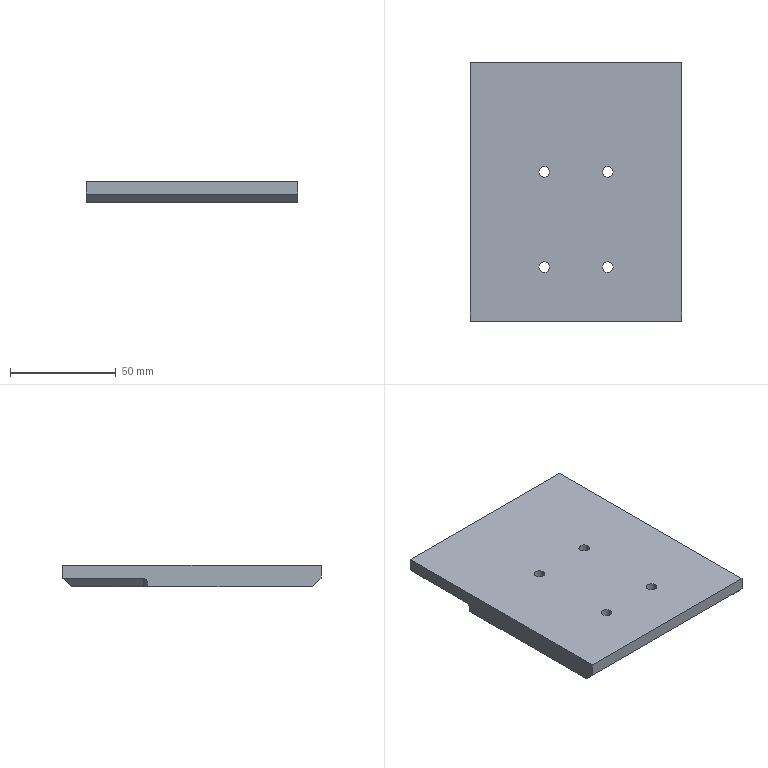Part | STEP file | X77-02102 | 1 solid | 30 faces | box 100 x 122 x 10 mm | volume 118906 mm3 | cylinder 14 | plane 12 | cone 4 | commonest cylinder face diameters 5 x8 4.2 x4 4 x2
STEP:
#1=CARTESIAN_POINT('',(17.5,9.5,10.));
#2=VERTEX_POINT('',#1);
#3=CARTESIAN_POINT('',(12.5,9.5,10.));
#4=VERTEX_POINT('',#3);
#5=CARTESIAN_POINT('',(15.,9.5,10.));
#6=DIRECTION('',(0.,0.,-1.));
#7=DIRECTION('',(-1.,0.,0.));
#8=AXIS2_PLACEMENT_3D('',#5,#6,#7);
#9=CIRCLE('',#8,2.5);
#10=EDGE_CURVE('',#2,#4,#9,.T.);
#11=ORIENTED_EDGE('',*,*,#10,.F.);
#12=CARTESIAN_POINT('',(17.5,9.5,0.));
#13=VERTEX_POINT('',#12);
#14=CARTESIAN_POINT('',(17.5,9.5,0.));
#15=DIRECTION('',(0.,0.,-1.));
#16=VECTOR('',#15,1000.);
#17=LINE('',#14,#16);
#18=EDGE_CURVE('',#2,#13,#17,.T.);
#19=ORIENTED_EDGE('',*,*,#18,.T.);
#20=CARTESIAN_POINT('',(12.5,9.5,0.));
#21=VERTEX_POINT('',#20);
#22=CARTESIAN_POINT('',(15.,9.5,0.));
#23=DIRECTION('',(0.,0.,-1.));
#24=DIRECTION('',(-1.,0.,0.));
#25=AXIS2_PLACEMENT_3D('',#22,#23,#24);
#26=CIRCLE('',#25,2.5);
#27=EDGE_CURVE('',#13,#21,#26,.T.);
#28=ORIENTED_EDGE('',*,*,#27,.T.);
#29=CARTESIAN_POINT('',(12.5,9.5,0.));
#30=DIRECTION('',(0.,0.,-1.));
#31=VECTOR('',#30,1000.);
#32=LINE('',#29,#31);
#33=EDGE_CURVE('',#4,#21,#32,.T.);
#34=ORIENTED_EDGE('',*,*,#33,.F.);
#35=EDGE_LOOP('',(#11,#19,#28,#34));
#36=FACE_OUTER_BOUND('',#35,.T.);
#37=CARTESIAN_POINT('',(15.,9.5,0.));
#38=DIRECTION('',(0.,0.,-1.));
#39=DIRECTION('',(-1.,0.,0.));
#40=AXIS2_PLACEMENT_3D('',#37,#38,#39);
#41=CYLINDRICAL_SURFACE('',#40,2.5);
#42=ADVANCED_FACE('',(#36),#41,.F.);
#43=CARTESIAN_POINT('',(17.5,-35.5,10.));
#44=VERTEX_POINT('',#43);
#45=CARTESIAN_POINT('',(12.5,-35.5,10.));
#46=VERTEX_POINT('',#45);
#47=CARTESIAN_POINT('',(15.,-35.5,10.));
#48=DIRECTION('',(0.,0.,-1.));
#49=DIRECTION('',(-1.,0.,0.));
#50=AXIS2_PLACEMENT_3D('',#47,#48,#49);
#51=CIRCLE('',#50,2.5);
#52=EDGE_CURVE('',#44,#46,#51,.T.);
#53=ORIENTED_EDGE('',*,*,#52,.F.);
#54=CARTESIAN_POINT('',(17.5,-35.5,0.));
#55=VERTEX_POINT('',#54);
#56=CARTESIAN_POINT('',(17.5,-35.5,0.));
#57=DIRECTION('',(0.,0.,-1.));
#58=VECTOR('',#57,1000.);
#59=LINE('',#56,#58);
#60=EDGE_CURVE('',#44,#55,#59,.T.);
#61=ORIENTED_EDGE('',*,*,#60,.T.);
#62=CARTESIAN_POINT('',(12.5,-35.5,0.));
#63=VERTEX_POINT('',#62);
#64=CARTESIAN_POINT('',(15.,-35.5,0.));
#65=DIRECTION('',(0.,0.,-1.));
#66=DIRECTION('',(-1.,0.,0.));
#67=AXIS2_PLACEMENT_3D('',#64,#65,#66);
#68=CIRCLE('',#67,2.5);
#69=EDGE_CURVE('',#55,#63,#68,.T.);
#70=ORIENTED_EDGE('',*,*,#69,.T.);
#71=CARTESIAN_POINT('',(12.5,-35.5,0.));
#72=DIRECTION('',(0.,0.,-1.));
#73=VECTOR('',#72,1000.);
#74=LINE('',#71,#73);
#75=EDGE_CURVE('',#46,#63,#74,.T.);
#76=ORIENTED_EDGE('',*,*,#75,.F.);
#77=EDGE_LOOP('',(#53,#61,#70,#76));
#78=FACE_OUTER_BOUND('',#77,.T.);
#79=CARTESIAN_POINT('',(15.,-35.5,0.));
#80=DIRECTION('',(0.,0.,-1.));
#81=DIRECTION('',(-1.,0.,0.));
#82=AXIS2_PLACEMENT_3D('',#79,#80,#81);
#83=CYLINDRICAL_SURFACE('',#82,2.5);
#84=ADVANCED_FACE('',(#78),#83,.F.);
#85=CARTESIAN_POINT('',(-12.5,-35.5,10.));
#86=VERTEX_POINT('',#85);
#87=CARTESIAN_POINT('',(-17.5,-35.5,10.));
#88=VERTEX_POINT('',#87);
#89=CARTESIAN_POINT('',(-15.,-35.5,10.));
#90=DIRECTION('',(0.,0.,-1.));
#91=DIRECTION('',(-1.,0.,0.));
#92=AXIS2_PLACEMENT_3D('',#89,#90,#91);
#93=CIRCLE('',#92,2.5);
#94=EDGE_CURVE('',#86,#88,#93,.T.);
#95=ORIENTED_EDGE('',*,*,#94,.F.);
#96=CARTESIAN_POINT('',(-12.5,-35.5,0.));
#97=VERTEX_POINT('',#96);
#98=CARTESIAN_POINT('',(-12.5,-35.5,0.));
#99=DIRECTION('',(0.,0.,-1.));
#100=VECTOR('',#99,1000.);
#101=LINE('',#98,#100);
#102=EDGE_CURVE('',#86,#97,#101,.T.);
#103=ORIENTED_EDGE('',*,*,#102,.T.);
#104=CARTESIAN_POINT('',(-17.5,-35.5,0.));
#105=VERTEX_POINT('',#104);
#106=CARTESIAN_POINT('',(-15.,-35.5,0.));
#107=DIRECTION('',(0.,0.,-1.));
#108=DIRECTION('',(-1.,0.,0.));
#109=AXIS2_PLACEMENT_3D('',#106,#107,#108);
#110=CIRCLE('',#109,2.5);
#111=EDGE_CURVE('',#97,#105,#110,.T.);
#112=ORIENTED_EDGE('',*,*,#111,.T.);
#113=CARTESIAN_POINT('',(-17.5,-35.5,0.));
#114=DIRECTION('',(0.,0.,-1.));
#115=VECTOR('',#114,1000.);
#116=LINE('',#113,#115);
#117=EDGE_CURVE('',#88,#105,#116,.T.);
#118=ORIENTED_EDGE('',*,*,#117,.F.);
#119=EDGE_LOOP('',(#95,#103,#112,#118));
#120=FACE_OUTER_BOUND('',#119,.T.);
#121=CARTESIAN_POINT('',(-15.,-35.5,0.));
#122=DIRECTION('',(0.,0.,-1.));
#123=DIRECTION('',(-1.,0.,0.));
#124=AXIS2_PLACEMENT_3D('',#121,#122,#123);
#125=CYLINDRICAL_SURFACE('',#124,2.5);
#126=ADVANCED_FACE('',(#120),#125,.F.);
#127=CARTESIAN_POINT('',(-12.5,9.5,10.));
#128=VERTEX_POINT('',#127);
#129=CARTESIAN_POINT('',(-17.5,9.5,10.));
#130=VERTEX_POINT('',#129);
#131=CARTESIAN_POINT('',(-15.,9.5,10.));
#132=DIRECTION('',(0.,0.,-1.));
#133=DIRECTION('',(-1.,0.,0.));
#134=AXIS2_PLACEMENT_3D('',#131,#132,#133);
#135=CIRCLE('',#134,2.5);
#136=EDGE_CURVE('',#128,#130,#135,.T.);
#137=ORIENTED_EDGE('',*,*,#136,.F.);
#138=CARTESIAN_POINT('',(-12.5,9.5,0.));
#139=VERTEX_POINT('',#138);
#140=CARTESIAN_POINT('',(-12.5,9.5,0.));
#141=DIRECTION('',(0.,0.,-1.));
#142=VECTOR('',#141,1000.);
#143=LINE('',#140,#142);
#144=EDGE_CURVE('',#128,#139,#143,.T.);
#145=ORIENTED_EDGE('',*,*,#144,.T.);
#146=CARTESIAN_POINT('',(-17.5,9.5,0.));
#147=VERTEX_POINT('',#146);
#148=CARTESIAN_POINT('',(-15.,9.5,0.));
#149=DIRECTION('',(0.,0.,-1.));
#150=DIRECTION('',(-1.,0.,0.));
#151=AXIS2_PLACEMENT_3D('',#148,#149,#150);
#152=CIRCLE('',#151,2.5);
#153=EDGE_CURVE('',#139,#147,#152,.T.);
#154=ORIENTED_EDGE('',*,*,#153,.T.);
#155=CARTESIAN_POINT('',(-17.5,9.5,0.));
#156=DIRECTION('',(0.,0.,-1.));
#157=VECTOR('',#156,1000.);
#158=LINE('',#155,#157);
#159=EDGE_CURVE('',#130,#147,#158,.T.);
#160=ORIENTED_EDGE('',*,*,#159,.F.);
#161=EDGE_LOOP('',(#137,#145,#154,#160));
#162=FACE_OUTER_BOUND('',#161,.T.);
#163=CARTESIAN_POINT('',(-15.,9.5,0.));
#164=DIRECTION('',(0.,0.,-1.));
#165=DIRECTION('',(-1.,0.,0.));
#166=AXIS2_PLACEMENT_3D('',#163,#164,#165);
#167=CYLINDRICAL_SURFACE('',#166,2.5);
#168=ADVANCED_FACE('',(#162),#167,.F.);
#169=CARTESIAN_POINT('',(32.1,41.,3.9));
#170=VERTEX_POINT('',#169);
#171=CARTESIAN_POINT('',(27.9,41.,3.9));
#172=VERTEX_POINT('',#171);
#173=CARTESIAN_POINT('',(30.,41.,3.9));
#174=DIRECTION('',(0.,0.,-1.));
#175=DIRECTION('',(-1.,0.,0.));
#176=AXIS2_PLACEMENT_3D('',#173,#174,#175);
#177=CIRCLE('',#176,2.1);
#178=EDGE_CURVE('',#170,#172,#177,.T.);
#179=ORIENTED_EDGE('',*,*,#178,.F.);
#180=CARTESIAN_POINT('',(32.1,41.,0.));
#181=VERTEX_POINT('',#180);
#182=CARTESIAN_POINT('',(32.1,41.,-8.5));
#183=DIRECTION('',(0.,0.,-1.));
#184=VECTOR('',#183,1000.);
#185=LINE('',#182,#184);
#186=EDGE_CURVE('',#170,#181,#185,.T.);
#187=ORIENTED_EDGE('',*,*,#186,.T.);
#188=CARTESIAN_POINT('',(27.9,41.,0.));
#189=VERTEX_POINT('',#188);
#190=CARTESIAN_POINT('',(30.,41.,0.));
#191=DIRECTION('',(0.,0.,-1.));
#192=DIRECTION('',(-1.,0.,0.));
#193=AXIS2_PLACEMENT_3D('',#190,#191,#192);
#194=CIRCLE('',#193,2.1);
#195=EDGE_CURVE('',#181,#189,#194,.T.);
#196=ORIENTED_EDGE('',*,*,#195,.T.);
#197=CARTESIAN_POINT('',(27.9,41.,-8.5));
#198=DIRECTION('',(0.,0.,-1.));
#199=VECTOR('',#198,1000.);
#200=LINE('',#197,#199);
#201=EDGE_CURVE('',#172,#189,#200,.T.);
#202=ORIENTED_EDGE('',*,*,#201,.F.);
#203=EDGE_LOOP('',(#179,#187,#196,#202));
#204=FACE_OUTER_BOUND('',#203,.T.);
#205=CARTESIAN_POINT('',(30.,41.,-8.5));
#206=DIRECTION('',(0.,0.,-1.));
#207=DIRECTION('',(-1.,0.,0.));
#208=AXIS2_PLACEMENT_3D('',#205,#206,#207);
#209=CYLINDRICAL_SURFACE('',#208,2.1);
#210=ADVANCED_FACE('',(#204),#209,.F.);
#211=CARTESIAN_POINT('',(30.,41.,5.162));
#212=VERTEX_POINT('',#211);
#213=CARTESIAN_POINT('',(27.9,41.,3.9));
#214=DIRECTION('',(-0.8572,0.,-0.515));
#215=VECTOR('',#214,1000.);
#216=LINE('',#213,#215);
#217=EDGE_CURVE('',#212,#172,#216,.T.);
#218=ORIENTED_EDGE('',*,*,#217,.F.);
#219=CARTESIAN_POINT('',(32.1,41.,3.9));
#220=DIRECTION('',(0.8572,0.,-0.515));
#221=VECTOR('',#220,1000.);
#222=LINE('',#219,#221);
#223=EDGE_CURVE('',#212,#170,#222,.T.);
#224=ORIENTED_EDGE('',*,*,#223,.T.);
#225=ORIENTED_EDGE('',*,*,#178,.T.);
#226=EDGE_LOOP('',(#218,#224,#225));
#227=FACE_OUTER_BOUND('',#226,.T.);
#228=CARTESIAN_POINT('',(30.,41.,3.9));
#229=DIRECTION('',(0.,0.,-1.));
#230=DIRECTION('',(-1.,0.,0.));
#231=AXIS2_PLACEMENT_3D('',#228,#229,#230);
#232=CONICAL_SURFACE('',#231,2.1,1.03);
#233=ADVANCED_FACE('',(#227),#232,.F.);
#234=CARTESIAN_POINT('',(-27.9,41.,3.9));
#235=VERTEX_POINT('',#234);
#236=CARTESIAN_POINT('',(-32.1,41.,3.9));
#237=VERTEX_POINT('',#236);
#238=CARTESIAN_POINT('',(-30.,41.,3.9));
#239=DIRECTION('',(0.,0.,-1.));
#240=DIRECTION('',(-1.,0.,0.));
#241=AXIS2_PLACEMENT_3D('',#238,#239,#240);
#242=CIRCLE('',#241,2.1);
#243=EDGE_CURVE('',#235,#237,#242,.T.);
#244=ORIENTED_EDGE('',*,*,#243,.F.);
#245=CARTESIAN_POINT('',(-27.9,41.,0.));
#246=VERTEX_POINT('',#245);
#247=CARTESIAN_POINT('',(-27.9,41.,-8.5));
#248=DIRECTION('',(0.,0.,-1.));
#249=VECTOR('',#248,1000.);
#250=LINE('',#247,#249);
#251=EDGE_CURVE('',#235,#246,#250,.T.);
#252=ORIENTED_EDGE('',*,*,#251,.T.);
#253=CARTESIAN_POINT('',(-32.1,41.,0.));
#254=VERTEX_POINT('',#253);
#255=CARTESIAN_POINT('',(-30.,41.,0.));
#256=DIRECTION('',(0.,0.,-1.));
#257=DIRECTION('',(-1.,0.,0.));
#258=AXIS2_PLACEMENT_3D('',#255,#256,#257);
#259=CIRCLE('',#258,2.1);
#260=EDGE_CURVE('',#246,#254,#259,.T.);
#261=ORIENTED_EDGE('',*,*,#260,.T.);
#262=CARTESIAN_POINT('',(-32.1,41.,-8.5));
#263=DIRECTION('',(0.,0.,-1.));
#264=VECTOR('',#263,1000.);
#265=LINE('',#262,#264);
#266=EDGE_CURVE('',#237,#254,#265,.T.);
#267=ORIENTED_EDGE('',*,*,#266,.F.);
#268=EDGE_LOOP('',(#244,#252,#261,#267));
#269=FACE_OUTER_BOUND('',#268,.T.);
#270=CARTESIAN_POINT('',(-30.,41.,-8.5));
#271=DIRECTION('',(0.,0.,-1.));
#272=DIRECTION('',(-1.,0.,0.));
#273=AXIS2_PLACEMENT_3D('',#270,#271,#272);
#274=CYLINDRICAL_SURFACE('',#273,2.1);
#275=ADVANCED_FACE('',(#269),#274,.F.);
#276=CARTESIAN_POINT('',(-30.,41.,5.162));
#277=VERTEX_POINT('',#276);
#278=CARTESIAN_POINT('',(-32.1,41.,3.9));
#279=DIRECTION('',(-0.8572,0.,-0.515));
#280=VECTOR('',#279,1000.);
#281=LINE('',#278,#280);
#282=EDGE_CURVE('',#277,#237,#281,.T.);
#283=ORIENTED_EDGE('',*,*,#282,.F.);
#284=CARTESIAN_POINT('',(-27.9,41.,3.9));
#285=DIRECTION('',(0.8572,0.,-0.515));
#286=VECTOR('',#285,1000.);
#287=LINE('',#284,#286);
#288=EDGE_CURVE('',#277,#235,#287,.T.);
#289=ORIENTED_EDGE('',*,*,#288,.T.);
#290=ORIENTED_EDGE('',*,*,#243,.T.);
#291=EDGE_LOOP('',(#283,#289,#290));
#292=FACE_OUTER_BOUND('',#291,.T.);
#293=CARTESIAN_POINT('',(-30.,41.,3.9));
#294=DIRECTION('',(0.,0.,-1.));
#295=DIRECTION('',(-1.,0.,0.));
#296=AXIS2_PLACEMENT_3D('',#293,#294,#295);
#297=CONICAL_SURFACE('',#296,2.1,1.03);
#298=ADVANCED_FACE('',(#292),#297,.F.);
#299=CARTESIAN_POINT('',(50.,-61.,10.));
#300=VERTEX_POINT('',#299);
#301=CARTESIAN_POINT('',(50.,-61.,4.));
#302=VERTEX_POINT('',#301);
#303=CARTESIAN_POINT('',(50.,-61.,10.));
#304=DIRECTION('',(0.,0.,-1.));
#305=VECTOR('',#304,1000.);
#306=LINE('',#303,#305);
#307=EDGE_CURVE('',#300,#302,#306,.T.);
#308=ORIENTED_EDGE('',*,*,#307,.T.);
#309=CARTESIAN_POINT('',(50.,-57.,0.));
#310=VERTEX_POINT('',#309);
#311=CARTESIAN_POINT('',(50.,-61.,4.));
#312=DIRECTION('',(0.,0.7071,-0.7071));
#313=VECTOR('',#312,1000.);
#314=LINE('',#311,#313);
#315=EDGE_CURVE('',#302,#310,#314,.T.);
#316=ORIENTED_EDGE('',*,*,#315,.T.);
#317=CARTESIAN_POINT('',(50.,21.,0.));
#318=VERTEX_POINT('',#317);
#319=CARTESIAN_POINT('',(50.,-61.,0.));
#320=DIRECTION('',(0.,1.,0.));
#321=VECTOR('',#320,1000.);
#322=LINE('',#319,#321);
#323=EDGE_CURVE('',#310,#318,#322,.T.);
#324=ORIENTED_EDGE('',*,*,#323,.T.);
#325=CARTESIAN_POINT('',(50.,21.,1.172));
#326=VERTEX_POINT('',#325);
#327=CARTESIAN_POINT('',(50.,21.,4.));
#328=DIRECTION('',(0.,0.,-1.));
#329=VECTOR('',#328,1000.);
#330=LINE('',#327,#329);
#331=EDGE_CURVE('',#326,#318,#330,.T.);
#332=ORIENTED_EDGE('',*,*,#331,.F.);
#333=CARTESIAN_POINT('',(50.,23.,4.));
#334=VERTEX_POINT('',#333);
#335=CARTESIAN_POINT('',(50.,21.,1.172));
#336=CARTESIAN_POINT('',(50.,21.,2.828));
#337=CARTESIAN_POINT('',(50.,21.828,4.));
#338=CARTESIAN_POINT('',(50.,23.,4.));
#339=(BOUNDED_CURVE()B_SPLINE_CURVE(3,(#335,#336,#337,#338),.UNSPECIFIED.,.F.,.F.)B_SPLINE_CURVE_WITH_KNOTS((4,4),(4.712,6.283),.UNSPECIFIED.)CURVE()GEOMETRIC_REPRESENTATION_ITEM()RATIONAL_B_SPLINE_CURVE((1.,0.8047,0.8047,1.))REPRESENTATION_ITEM(''));
#340=EDGE_CURVE('',#326,#334,#339,.T.);
#341=ORIENTED_EDGE('',*,*,#340,.T.);
#342=CARTESIAN_POINT('',(50.,61.,4.));
#343=VERTEX_POINT('',#342);
#344=CARTESIAN_POINT('',(50.,21.,4.));
#345=DIRECTION('',(0.,1.,0.));
#346=VECTOR('',#345,1000.);
#347=LINE('',#344,#346);
#348=EDGE_CURVE('',#334,#343,#347,.T.);
#349=ORIENTED_EDGE('',*,*,#348,.T.);
#350=CARTESIAN_POINT('',(50.,61.,10.));
#351=VERTEX_POINT('',#350);
#352=CARTESIAN_POINT('',(50.,61.,10.));
#353=DIRECTION('',(0.,0.,-1.));
#354=VECTOR('',#353,1000.);
#355=LINE('',#352,#354);
#356=EDGE_CURVE('',#351,#343,#355,.T.);
#357=ORIENTED_EDGE('',*,*,#356,.F.);
#358=CARTESIAN_POINT('',(50.,-61.,10.));
#359=DIRECTION('',(0.,1.,0.));
#360=VECTOR('',#359,1000.);
#361=LINE('',#358,#360);
#362=EDGE_CURVE('',#300,#351,#361,.T.);
#363=ORIENTED_EDGE('',*,*,#362,.F.);
#364=EDGE_LOOP('',(#308,#316,#324,#332,#341,#349,#357,#363));
#365=FACE_OUTER_BOUND('',#364,.T.);
#366=CARTESIAN_POINT('',(50.,-61.,10.));
#367=DIRECTION('',(-1.,0.,0.));
#368=DIRECTION('',(0.,0.,1.));
#369=AXIS2_PLACEMENT_3D('',#366,#367,#368);
#370=PLANE('',#369);
#371=ADVANCED_FACE('',(#365),#370,.F.);
#372=ORIENTED_EDGE('',*,*,#356,.T.);
#373=CARTESIAN_POINT('',(-50.,61.,4.));
#374=VERTEX_POINT('',#373);
#375=CARTESIAN_POINT('',(-50.,61.,4.));
#376=DIRECTION('',(-1.,0.,0.));
#377=VECTOR('',#376,1000.);
#378=LINE('',#375,#377);
#379=EDGE_CURVE('',#343,#374,#378,.T.);
#380=ORIENTED_EDGE('',*,*,#379,.T.);
#381=CARTESIAN_POINT('',(-50.,61.,10.));
#382=VERTEX_POINT('',#381);
#383=CARTESIAN_POINT('',(-50.,61.,10.));
#384=DIRECTION('',(0.,0.,-1.));
#385=VECTOR('',#384,1000.);
#386=LINE('',#383,#385);
#387=EDGE_CURVE('',#382,#374,#386,.T.);
#388=ORIENTED_EDGE('',*,*,#387,.F.);
#389=CARTESIAN_POINT('',(-50.,61.,10.));
#390=DIRECTION('',(-1.,0.,0.));
#391=VECTOR('',#390,1000.);
#392=LINE('',#389,#391);
#393=EDGE_CURVE('',#351,#382,#392,.T.);
#394=ORIENTED_EDGE('',*,*,#393,.F.);
#395=EDGE_LOOP('',(#372,#380,#388,#394));
#396=FACE_OUTER_BOUND('',#395,.T.);
#397=CARTESIAN_POINT('',(-50.,61.,10.));
#398=DIRECTION('',(0.,-1.,0.));
#399=DIRECTION('',(0.,0.,-1.));
#400=AXIS2_PLACEMENT_3D('',#397,#398,#399);
#401=PLANE('',#400);
#402=ADVANCED_FACE('',(#396),#401,.F.);
#403=CARTESIAN_POINT('',(-50.,21.,0.));
#404=VERTEX_POINT('',#403);
#405=CARTESIAN_POINT('',(-50.,-57.,0.));
#406=VERTEX_POINT('',#405);
#407=CARTESIAN_POINT('',(-50.,-61.,0.));
#408=DIRECTION('',(0.,-1.,0.));
#409=VECTOR('',#408,1000.);
#410=LINE('',#407,#409);
#411=EDGE_CURVE('',#404,#406,#410,.T.);
#412=ORIENTED_EDGE('',*,*,#411,.T.);
#413=CARTESIAN_POINT('',(-50.,-61.,4.));
#414=VERTEX_POINT('',#413);
#415=CARTESIAN_POINT('',(-50.,-61.,4.));
#416=DIRECTION('',(0.,-0.7071,0.7071));
#417=VECTOR('',#416,1000.);
#418=LINE('',#415,#417);
#419=EDGE_CURVE('',#406,#414,#418,.T.);
#420=ORIENTED_EDGE('',*,*,#419,.T.);
#421=CARTESIAN_POINT('',(-50.,-61.,10.));
#422=VERTEX_POINT('',#421);
#423=CARTESIAN_POINT('',(-50.,-61.,10.));
#424=DIRECTION('',(0.,0.,-1.));
#425=VECTOR('',#424,1000.);
#426=LINE('',#423,#425);
#427=EDGE_CURVE('',#422,#414,#426,.T.);
#428=ORIENTED_EDGE('',*,*,#427,.F.);
#429=CARTESIAN_POINT('',(-50.,-61.,10.));
#430=DIRECTION('',(0.,-1.,0.));
#431=VECTOR('',#430,1000.);
#432=LINE('',#429,#431);
#433=EDGE_CURVE('',#382,#422,#432,.T.);
#434=ORIENTED_EDGE('',*,*,#433,.F.);
#435=ORIENTED_EDGE('',*,*,#387,.T.);
#436=CARTESIAN_POINT('',(-50.,23.,4.));
#437=VERTEX_POINT('',#436);
#438=CARTESIAN_POINT('',(-50.,21.,4.));
#439=DIRECTION('',(0.,1.,0.));
#440=VECTOR('',#439,1000.);
#441=LINE('',#438,#440);
#442=EDGE_CURVE('',#437,#374,#441,.T.);
#443=ORIENTED_EDGE('',*,*,#442,.F.);
#444=CARTESIAN_POINT('',(-50.,21.,1.172));
#445=VERTEX_POINT('',#444);
#446=CARTESIAN_POINT('',(-50.,23.,4.));
#447=CARTESIAN_POINT('',(-50.,21.828,4.));
#448=CARTESIAN_POINT('',(-50.,21.,2.828));
#449=CARTESIAN_POINT('',(-50.,21.,1.172));
#450=(BOUNDED_CURVE()B_SPLINE_CURVE(3,(#446,#447,#448,#449),.UNSPECIFIED.,.F.,.F.)B_SPLINE_CURVE_WITH_KNOTS((4,4),(0.,1.571),.UNSPECIFIED.)CURVE()GEOMETRIC_REPRESENTATION_ITEM()RATIONAL_B_SPLINE_CURVE((1.,0.8047,0.8047,1.))REPRESENTATION_ITEM(''));
#451=EDGE_CURVE('',#437,#445,#450,.T.);
#452=ORIENTED_EDGE('',*,*,#451,.T.);
#453=CARTESIAN_POINT('',(-50.,21.,0.));
#454=DIRECTION('',(0.,0.,1.));
#455=VECTOR('',#454,1000.);
#456=LINE('',#453,#455);
#457=EDGE_CURVE('',#404,#445,#456,.T.);
#458=ORIENTED_EDGE('',*,*,#457,.F.);
#459=EDGE_LOOP('',(#412,#420,#428,#434,#435,#443,#452,#458));
#460=FACE_OUTER_BOUND('',#459,.T.);
#461=CARTESIAN_POINT('',(-50.,-61.,10.));
#462=DIRECTION('',(1.,0.,0.));
#463=DIRECTION('',(0.,0.,-1.));
#464=AXIS2_PLACEMENT_3D('',#461,#462,#463);
#465=PLANE('',#464);
#466=ADVANCED_FACE('',(#460),#465,.F.);
#467=ORIENTED_EDGE('',*,*,#427,.T.);
#468=CARTESIAN_POINT('',(50.,-61.,4.));
#469=DIRECTION('',(1.,0.,0.));
#470=VECTOR('',#469,1000.);
#471=LINE('',#468,#470);
#472=EDGE_CURVE('',#414,#302,#471,.T.);
#473=ORIENTED_EDGE('',*,*,#472,.T.);
#474=ORIENTED_EDGE('',*,*,#307,.F.);
#475=CARTESIAN_POINT('',(-50.,-61.,10.));
#476=DIRECTION('',(1.,0.,0.));
#477=VECTOR('',#476,1000.);
#478=LINE('',#475,#477);
#479=EDGE_CURVE('',#422,#300,#478,.T.);
#480=ORIENTED_EDGE('',*,*,#479,.F.);
#481=EDGE_LOOP('',(#467,#473,#474,#480));
#482=FACE_OUTER_BOUND('',#481,.T.);
#483=CARTESIAN_POINT('',(-50.,-61.,10.));
#484=DIRECTION('',(0.,1.,0.));
#485=DIRECTION('',(0.,0.,1.));
#486=AXIS2_PLACEMENT_3D('',#483,#484,#485);
#487=PLANE('',#486);
#488=ADVANCED_FACE('',(#482),#487,.F.);
#489=CARTESIAN_POINT('',(15.,9.5,10.));
#490=DIRECTION('',(0.,0.,-1.));
#491=DIRECTION('',(-1.,0.,0.));
#492=AXIS2_PLACEMENT_3D('',#489,#490,#491);
#493=CIRCLE('',#492,2.5);
#494=EDGE_CURVE('',#4,#2,#493,.T.);
#495=ORIENTED_EDGE('',*,*,#494,.T.);
#496=ORIENTED_EDGE('',*,*,#10,.T.);
#497=EDGE_LOOP('',(#495,#496));
#498=FACE_BOUND('',#497,.T.);
#499=CARTESIAN_POINT('',(15.,-35.5,10.));
#500=DIRECTION('',(0.,0.,-1.));
#501=DIRECTION('',(-1.,0.,0.));
#502=AXIS2_PLACEMENT_3D('',#499,#500,#501);
#503=CIRCLE('',#502,2.5);
#504=EDGE_CURVE('',#46,#44,#503,.T.);
#505=ORIENTED_EDGE('',*,*,#504,.T.);
#506=ORIENTED_EDGE('',*,*,#52,.T.);
#507=EDGE_LOOP('',(#505,#506));
#508=FACE_BOUND('',#507,.T.);
#509=CARTESIAN_POINT('',(-15.,-35.5,10.));
#510=DIRECTION('',(0.,0.,-1.));
#511=DIRECTION('',(-1.,0.,0.));
#512=AXIS2_PLACEMENT_3D('',#509,#510,#511);
#513=CIRCLE('',#512,2.5);
#514=EDGE_CURVE('',#88,#86,#513,.T.);
#515=ORIENTED_EDGE('',*,*,#514,.T.);
#516=ORIENTED_EDGE('',*,*,#94,.T.);
#517=EDGE_LOOP('',(#515,#516));
#518=FACE_BOUND('',#517,.T.);
#519=CARTESIAN_POINT('',(-15.,9.5,10.));
#520=DIRECTION('',(0.,0.,-1.));
#521=DIRECTION('',(-1.,0.,0.));
#522=AXIS2_PLACEMENT_3D('',#519,#520,#521);
#523=CIRCLE('',#522,2.5);
#524=EDGE_CURVE('',#130,#128,#523,.T.);
#525=ORIENTED_EDGE('',*,*,#524,.T.);
#526=ORIENTED_EDGE('',*,*,#136,.T.);
#527=EDGE_LOOP('',(#525,#526));
#528=FACE_BOUND('',#527,.T.);
#529=ORIENTED_EDGE('',*,*,#362,.T.);
#530=ORIENTED_EDGE('',*,*,#393,.T.);
#531=ORIENTED_EDGE('',*,*,#433,.T.);
#532=ORIENTED_EDGE('',*,*,#479,.T.);
#533=EDGE_LOOP('',(#529,#530,#531,#532));
#534=FACE_OUTER_BOUND('',#533,.T.);
#535=CARTESIAN_POINT('',(50.,61.,10.));
#536=DIRECTION('',(0.,0.,-1.));
#537=DIRECTION('',(-1.,0.,0.));
#538=AXIS2_PLACEMENT_3D('',#535,#536,#537);
#539=PLANE('',#538);
#540=ADVANCED_FACE('',(#498,#508,#518,#528,#534),#539,.F.);
#541=CARTESIAN_POINT('',(15.,9.5,0.));
#542=DIRECTION('',(0.,0.,-1.));
#543=DIRECTION('',(-1.,0.,0.));
#544=AXIS2_PLACEMENT_3D('',#541,#542,#543);
#545=CIRCLE('',#544,2.5);
#546=EDGE_CURVE('',#21,#13,#545,.T.);
#547=ORIENTED_EDGE('',*,*,#546,.F.);
#548=ORIENTED_EDGE('',*,*,#27,.F.);
#549=EDGE_LOOP('',(#547,#548));
#550=FACE_BOUND('',#549,.T.);
#551=CARTESIAN_POINT('',(15.,-35.5,0.));
#552=DIRECTION('',(0.,0.,-1.));
#553=DIRECTION('',(-1.,0.,0.));
#554=AXIS2_PLACEMENT_3D('',#551,#552,#553);
#555=CIRCLE('',#554,2.5);
#556=EDGE_CURVE('',#63,#55,#555,.T.);
#557=ORIENTED_EDGE('',*,*,#556,.F.);
#558=ORIENTED_EDGE('',*,*,#69,.F.);
#559=EDGE_LOOP('',(#557,#558));
#560=FACE_BOUND('',#559,.T.);
#561=CARTESIAN_POINT('',(-15.,-35.5,0.));
#562=DIRECTION('',(0.,0.,-1.));
#563=DIRECTION('',(-1.,0.,0.));
#564=AXIS2_PLACEMENT_3D('',#561,#562,#563);
#565=CIRCLE('',#564,2.5);
#566=EDGE_CURVE('',#105,#97,#565,.T.);
#567=ORIENTED_EDGE('',*,*,#566,.F.);
#568=ORIENTED_EDGE('',*,*,#111,.F.);
#569=EDGE_LOOP('',(#567,#568));
#570=FACE_BOUND('',#569,.T.);
#571=CARTESIAN_POINT('',(-15.,9.5,0.));
#572=DIRECTION('',(0.,0.,-1.));
#573=DIRECTION('',(-1.,0.,0.));
#574=AXIS2_PLACEMENT_3D('',#571,#572,#573);
#575=CIRCLE('',#574,2.5);
#576=EDGE_CURVE('',#147,#139,#575,.T.);
#577=ORIENTED_EDGE('',*,*,#576,.F.);
#578=ORIENTED_EDGE('',*,*,#153,.F.);
#579=EDGE_LOOP('',(#577,#578));
#580=FACE_BOUND('',#579,.T.);
#581=CARTESIAN_POINT('',(30.,41.,0.));
#582=DIRECTION('',(0.,0.,-1.));
#583=DIRECTION('',(-1.,0.,0.));
#584=AXIS2_PLACEMENT_3D('',#581,#582,#583);
#585=CIRCLE('',#584,2.1);
#586=EDGE_CURVE('',#189,#181,#585,.T.);
#587=ORIENTED_EDGE('',*,*,#586,.F.);
#588=ORIENTED_EDGE('',*,*,#195,.F.);
#589=EDGE_LOOP('',(#587,#588));
#590=FACE_BOUND('',#589,.T.);
#591=CARTESIAN_POINT('',(-30.,41.,0.));
#592=DIRECTION('',(0.,0.,-1.));
#593=DIRECTION('',(-1.,0.,0.));
#594=AXIS2_PLACEMENT_3D('',#591,#592,#593);
#595=CIRCLE('',#594,2.1);
#596=EDGE_CURVE('',#254,#246,#595,.T.);
#597=ORIENTED_EDGE('',*,*,#596,.F.);
#598=ORIENTED_EDGE('',*,*,#260,.F.);
#599=EDGE_LOOP('',(#597,#598));
#600=FACE_BOUND('',#599,.T.);
#601=ORIENTED_EDGE('',*,*,#323,.F.);
#602=CARTESIAN_POINT('',(-50.,-57.,0.));
#603=DIRECTION('',(-1.,0.,0.));
#604=VECTOR('',#603,1000.);
#605=LINE('',#602,#604);
#606=EDGE_CURVE('',#310,#406,#605,.T.);
#607=ORIENTED_EDGE('',*,*,#606,.T.);
#608=ORIENTED_EDGE('',*,*,#411,.F.);
#609=CARTESIAN_POINT('',(-48.828,21.,0.));
#610=VERTEX_POINT('',#609);
#611=CARTESIAN_POINT('',(-46.,21.,0.));
#612=DIRECTION('',(-1.,0.,0.));
#613=VECTOR('',#612,1000.);
#614=LINE('',#611,#613);
#615=EDGE_CURVE('',#610,#404,#614,.T.);
#616=ORIENTED_EDGE('',*,*,#615,.F.);
#617=CARTESIAN_POINT('',(-46.,23.,0.));
#618=VERTEX_POINT('',#617);
#619=CARTESIAN_POINT('',(-48.828,21.,0.));
#620=CARTESIAN_POINT('',(-47.172,21.,0.));
#621=CARTESIAN_POINT('',(-46.,21.828,0.));
#622=CARTESIAN_POINT('',(-46.,23.,0.));
#623=(BOUNDED_CURVE()B_SPLINE_CURVE(3,(#619,#620,#621,#622),.UNSPECIFIED.,.F.,.F.)B_SPLINE_CURVE_WITH_KNOTS((4,4),(1.571,3.142),.UNSPECIFIED.)CURVE()GEOMETRIC_REPRESENTATION_ITEM()RATIONAL_B_SPLINE_CURVE((1.,0.8047,0.8047,1.))REPRESENTATION_ITEM(''));
#624=EDGE_CURVE('',#610,#618,#623,.T.);
#625=ORIENTED_EDGE('',*,*,#624,.T.);
#626=CARTESIAN_POINT('',(-46.,57.,0.));
#627=VERTEX_POINT('',#626);
#628=CARTESIAN_POINT('',(-46.,21.,0.));
#629=DIRECTION('',(0.,1.,0.));
#630=VECTOR('',#629,1000.);
#631=LINE('',#628,#630);
#632=EDGE_CURVE('',#618,#627,#631,.T.);
#633=ORIENTED_EDGE('',*,*,#632,.T.);
#634=CARTESIAN_POINT('',(46.,57.,0.));
#635=VERTEX_POINT('',#634);
#636=CARTESIAN_POINT('',(50.,57.,0.));
#637=DIRECTION('',(1.,0.,0.));
#638=VECTOR('',#637,1000.);
#639=LINE('',#636,#638);
#640=EDGE_CURVE('',#627,#635,#639,.T.);
#641=ORIENTED_EDGE('',*,*,#640,.T.);
#642=CARTESIAN_POINT('',(46.,23.,0.));
#643=VERTEX_POINT('',#642);
#644=CARTESIAN_POINT('',(46.,21.,0.));
#645=DIRECTION('',(0.,1.,0.));
#646=VECTOR('',#645,1000.);
#647=LINE('',#644,#646);
#648=EDGE_CURVE('',#643,#635,#647,.T.);
#649=ORIENTED_EDGE('',*,*,#648,.F.);
#650=CARTESIAN_POINT('',(48.828,21.,0.));
#651=VERTEX_POINT('',#650);
#652=CARTESIAN_POINT('',(46.,23.,0.));
#653=CARTESIAN_POINT('',(46.,21.828,0.));
#654=CARTESIAN_POINT('',(47.172,21.,0.));
#655=CARTESIAN_POINT('',(48.828,21.,0.));
#656=(BOUNDED_CURVE()B_SPLINE_CURVE(3,(#652,#653,#654,#655),.UNSPECIFIED.,.F.,.F.)B_SPLINE_CURVE_WITH_KNOTS((4,4),(3.142,4.712),.UNSPECIFIED.)CURVE()GEOMETRIC_REPRESENTATION_ITEM()RATIONAL_B_SPLINE_CURVE((1.,0.8047,0.8047,1.))REPRESENTATION_ITEM(''));
#657=EDGE_CURVE('',#643,#651,#656,.T.);
#658=ORIENTED_EDGE('',*,*,#657,.T.);
#659=CARTESIAN_POINT('',(50.,21.,0.));
#660=DIRECTION('',(-1.,0.,0.));
#661=VECTOR('',#660,1000.);
#662=LINE('',#659,#661);
#663=EDGE_CURVE('',#318,#651,#662,.T.);
#664=ORIENTED_EDGE('',*,*,#663,.F.);
#665=EDGE_LOOP('',(#601,#607,#608,#616,#625,#633,#641,#649,#658,#664));
#666=FACE_OUTER_BOUND('',#665,.T.);
#667=CARTESIAN_POINT('',(50.,61.,0.));
#668=DIRECTION('',(0.,0.,-1.));
#669=DIRECTION('',(-1.,0.,0.));
#670=AXIS2_PLACEMENT_3D('',#667,#668,#669);
#671=PLANE('',#670);
#672=ADVANCED_FACE('',(#550,#560,#570,#580,#590,#600,#666),#671,.T.);
#673=CARTESIAN_POINT('',(16.667,27.667,-29.333));
#674=DIRECTION('',(0.5774,0.5774,0.5774));
#675=VECTOR('',#674,1000.);
#676=LINE('',#673,#675);
#677=EDGE_CURVE('',#635,#343,#676,.T.);
#678=ORIENTED_EDGE('',*,*,#677,.F.);
#679=ORIENTED_EDGE('',*,*,#640,.F.);
#680=CARTESIAN_POINT('',(-50.,61.,4.));
#681=DIRECTION('',(0.5774,-0.5774,-0.5774));
#682=VECTOR('',#681,1000.);
#683=LINE('',#680,#682);
#684=EDGE_CURVE('',#374,#627,#683,.T.);
#685=ORIENTED_EDGE('',*,*,#684,.F.);
#686=ORIENTED_EDGE('',*,*,#379,.F.);
#687=EDGE_LOOP('',(#678,#679,#685,#686));
#688=FACE_OUTER_BOUND('',#687,.T.);
#689=CARTESIAN_POINT('',(-50.,61.,4.));
#690=DIRECTION('',(0.,0.7071,-0.7071));
#691=DIRECTION('',(0.,0.7071,0.7071));
#692=AXIS2_PLACEMENT_3D('',#689,#690,#691);
#693=PLANE('',#692);
#694=ADVANCED_FACE('',(#688),#693,.T.);
#695=ORIENTED_EDGE('',*,*,#632,.F.);
#696=CARTESIAN_POINT('',(-50.,23.,4.));
#697=DIRECTION('',(-0.7071,0.,0.7071));
#698=VECTOR('',#697,1000.);
#699=LINE('',#696,#698);
#700=EDGE_CURVE('',#618,#437,#699,.T.);
#701=ORIENTED_EDGE('',*,*,#700,.T.);
#702=ORIENTED_EDGE('',*,*,#442,.T.);
#703=ORIENTED_EDGE('',*,*,#684,.T.);
#704=EDGE_LOOP('',(#695,#701,#702,#703));
#705=FACE_OUTER_BOUND('',#704,.T.);
#706=CARTESIAN_POINT('',(-50.,21.,4.));
#707=DIRECTION('',(0.7071,0.,0.7071));
#708=DIRECTION('',(0.7071,0.,-0.7071));
#709=AXIS2_PLACEMENT_3D('',#706,#707,#708);
#710=PLANE('',#709);
#711=ADVANCED_FACE('',(#705),#710,.F.);
#712=ORIENTED_EDGE('',*,*,#457,.T.);
#713=CARTESIAN_POINT('',(-47.414,21.,-1.414));
#714=DIRECTION('',(0.7071,0.,-0.7071));
#715=VECTOR('',#714,1000.);
#716=LINE('',#713,#715);
#717=EDGE_CURVE('',#445,#610,#716,.T.);
#718=ORIENTED_EDGE('',*,*,#717,.T.);
#719=ORIENTED_EDGE('',*,*,#615,.T.);
#720=EDGE_LOOP('',(#712,#718,#719));
#721=FACE_OUTER_BOUND('',#720,.T.);
#722=CARTESIAN_POINT('',(-50.,21.,0.));
#723=DIRECTION('',(0.,-1.,0.));
#724=DIRECTION('',(0.,0.,-1.));
#725=AXIS2_PLACEMENT_3D('',#722,#723,#724);
#726=PLANE('',#725);
#727=ADVANCED_FACE('',(#721),#726,.F.);
#728=ORIENTED_EDGE('',*,*,#348,.F.);
#729=CARTESIAN_POINT('',(46.,23.,0.));
#730=DIRECTION('',(-0.7071,0.,-0.7071));
#731=VECTOR('',#730,1000.);
#732=LINE('',#729,#731);
#733=EDGE_CURVE('',#334,#643,#732,.T.);
#734=ORIENTED_EDGE('',*,*,#733,.T.);
#735=ORIENTED_EDGE('',*,*,#648,.T.);
#736=ORIENTED_EDGE('',*,*,#677,.T.);
#737=EDGE_LOOP('',(#728,#734,#735,#736));
#738=FACE_OUTER_BOUND('',#737,.T.);
#739=CARTESIAN_POINT('',(46.,21.,0.));
#740=DIRECTION('',(-0.7071,0.,0.7071));
#741=DIRECTION('',(0.7071,0.,0.7071));
#742=AXIS2_PLACEMENT_3D('',#739,#740,#741);
#743=PLANE('',#742);
#744=ADVANCED_FACE('',(#738),#743,.F.);
#745=ORIENTED_EDGE('',*,*,#663,.T.);
#746=CARTESIAN_POINT('',(51.414,21.,2.586));
#747=DIRECTION('',(0.7071,0.,0.7071));
#748=VECTOR('',#747,1000.);
#749=LINE('',#746,#748);
#750=EDGE_CURVE('',#651,#326,#749,.T.);
#751=ORIENTED_EDGE('',*,*,#750,.T.);
#752=ORIENTED_EDGE('',*,*,#331,.T.);
#753=EDGE_LOOP('',(#745,#751,#752));
#754=FACE_OUTER_BOUND('',#753,.T.);
#755=CARTESIAN_POINT('',(50.,21.,4.));
#756=DIRECTION('',(0.,1.,0.));
#757=DIRECTION('',(0.,0.,1.));
#758=AXIS2_PLACEMENT_3D('',#755,#756,#757);
#759=PLANE('',#758);
#760=ADVANCED_FACE('',(#754),#759,.T.);
#761=ORIENTED_EDGE('',*,*,#451,.F.);
#762=ORIENTED_EDGE('',*,*,#700,.F.);
#763=ORIENTED_EDGE('',*,*,#624,.F.);
#764=ORIENTED_EDGE('',*,*,#717,.F.);
#765=EDGE_LOOP('',(#761,#762,#763,#764));
#766=FACE_OUTER_BOUND('',#765,.T.);
#767=CARTESIAN_POINT('',(-49.414,23.,0.5858));
#768=DIRECTION('',(-0.7071,0.,0.7071));
#769=DIRECTION('',(0.7071,0.,0.7071));
#770=AXIS2_PLACEMENT_3D('',#767,#768,#769);
#771=CYLINDRICAL_SURFACE('',#770,2.);
#772=ADVANCED_FACE('',(#766),#771,.F.);
#773=ORIENTED_EDGE('',*,*,#657,.F.);
#774=ORIENTED_EDGE('',*,*,#733,.F.);
#775=ORIENTED_EDGE('',*,*,#340,.F.);
#776=ORIENTED_EDGE('',*,*,#750,.F.);
#777=EDGE_LOOP('',(#773,#774,#775,#776));
#778=FACE_OUTER_BOUND('',#777,.T.);
#779=CARTESIAN_POINT('',(51.414,23.,2.586));
#780=DIRECTION('',(0.7071,0.,0.7071));
#781=DIRECTION('',(0.7071,0.,-0.7071));
#782=AXIS2_PLACEMENT_3D('',#779,#780,#781);
#783=CYLINDRICAL_SURFACE('',#782,2.);
#784=ADVANCED_FACE('',(#778),#783,.F.);
#785=ORIENTED_EDGE('',*,*,#419,.F.);
#786=ORIENTED_EDGE('',*,*,#606,.F.);
#787=ORIENTED_EDGE('',*,*,#315,.F.);
#788=ORIENTED_EDGE('',*,*,#472,.F.);
#789=EDGE_LOOP('',(#785,#786,#787,#788));
#790=FACE_OUTER_BOUND('',#789,.T.);
#791=CARTESIAN_POINT('',(-50.,-61.,4.));
#792=DIRECTION('',(0.,-0.7071,-0.7071));
#793=DIRECTION('',(0.,0.7071,-0.7071));
#794=AXIS2_PLACEMENT_3D('',#791,#792,#793);
#795=PLANE('',#794);
#796=ADVANCED_FACE('',(#790),#795,.T.);
#797=ORIENTED_EDGE('',*,*,#288,.F.);
#798=ORIENTED_EDGE('',*,*,#282,.T.);
#799=CARTESIAN_POINT('',(-30.,41.,3.9));
#800=DIRECTION('',(0.,0.,-1.));
#801=DIRECTION('',(-1.,0.,0.));
#802=AXIS2_PLACEMENT_3D('',#799,#800,#801);
#803=CIRCLE('',#802,2.1);
#804=EDGE_CURVE('',#237,#235,#803,.T.);
#805=ORIENTED_EDGE('',*,*,#804,.T.);
#806=EDGE_LOOP('',(#797,#798,#805));
#807=FACE_OUTER_BOUND('',#806,.T.);
#808=CARTESIAN_POINT('',(-30.,41.,3.9));
#809=DIRECTION('',(0.,0.,-1.));
#810=DIRECTION('',(-1.,0.,0.));
#811=AXIS2_PLACEMENT_3D('',#808,#809,#810);
#812=CONICAL_SURFACE('',#811,2.1,1.03);
#813=ADVANCED_FACE('',(#807),#812,.F.);
#814=ORIENTED_EDGE('',*,*,#251,.F.);
#815=ORIENTED_EDGE('',*,*,#804,.F.);
#816=ORIENTED_EDGE('',*,*,#266,.T.);
#817=ORIENTED_EDGE('',*,*,#596,.T.);
#818=EDGE_LOOP('',(#814,#815,#816,#817));
#819=FACE_OUTER_BOUND('',#818,.T.);
#820=CARTESIAN_POINT('',(-30.,41.,-8.5));
#821=DIRECTION('',(0.,0.,-1.));
#822=DIRECTION('',(-1.,0.,0.));
#823=AXIS2_PLACEMENT_3D('',#820,#821,#822);
#824=CYLINDRICAL_SURFACE('',#823,2.1);
#825=ADVANCED_FACE('',(#819),#824,.F.);
#826=ORIENTED_EDGE('',*,*,#223,.F.);
#827=ORIENTED_EDGE('',*,*,#217,.T.);
#828=CARTESIAN_POINT('',(30.,41.,3.9));
#829=DIRECTION('',(0.,0.,-1.));
#830=DIRECTION('',(-1.,0.,0.));
#831=AXIS2_PLACEMENT_3D('',#828,#829,#830);
#832=CIRCLE('',#831,2.1);
#833=EDGE_CURVE('',#172,#170,#832,.T.);
#834=ORIENTED_EDGE('',*,*,#833,.T.);
#835=EDGE_LOOP('',(#826,#827,#834));
#836=FACE_OUTER_BOUND('',#835,.T.);
#837=CARTESIAN_POINT('',(30.,41.,3.9));
#838=DIRECTION('',(0.,0.,-1.));
#839=DIRECTION('',(-1.,0.,0.));
#840=AXIS2_PLACEMENT_3D('',#837,#838,#839);
#841=CONICAL_SURFACE('',#840,2.1,1.03);
#842=ADVANCED_FACE('',(#836),#841,.F.);
#843=ORIENTED_EDGE('',*,*,#186,.F.);
#844=ORIENTED_EDGE('',*,*,#833,.F.);
#845=ORIENTED_EDGE('',*,*,#201,.T.);
#846=ORIENTED_EDGE('',*,*,#586,.T.);
#847=EDGE_LOOP('',(#843,#844,#845,#846));
#848=FACE_OUTER_BOUND('',#847,.T.);
#849=CARTESIAN_POINT('',(30.,41.,-8.5));
#850=DIRECTION('',(0.,0.,-1.));
#851=DIRECTION('',(-1.,0.,0.));
#852=AXIS2_PLACEMENT_3D('',#849,#850,#851);
#853=CYLINDRICAL_SURFACE('',#852,2.1);
#854=ADVANCED_FACE('',(#848),#853,.F.);
#855=ORIENTED_EDGE('',*,*,#144,.F.);
#856=ORIENTED_EDGE('',*,*,#524,.F.);
#857=ORIENTED_EDGE('',*,*,#159,.T.);
#858=ORIENTED_EDGE('',*,*,#576,.T.);
#859=EDGE_LOOP('',(#855,#856,#857,#858));
#860=FACE_OUTER_BOUND('',#859,.T.);
#861=CARTESIAN_POINT('',(-15.,9.5,0.));
#862=DIRECTION('',(0.,0.,-1.));
#863=DIRECTION('',(-1.,0.,0.));
#864=AXIS2_PLACEMENT_3D('',#861,#862,#863);
#865=CYLINDRICAL_SURFACE('',#864,2.5);
#866=ADVANCED_FACE('',(#860),#865,.F.);
#867=ORIENTED_EDGE('',*,*,#102,.F.);
#868=ORIENTED_EDGE('',*,*,#514,.F.);
#869=ORIENTED_EDGE('',*,*,#117,.T.);
#870=ORIENTED_EDGE('',*,*,#566,.T.);
#871=EDGE_LOOP('',(#867,#868,#869,#870));
#872=FACE_OUTER_BOUND('',#871,.T.);
#873=CARTESIAN_POINT('',(-15.,-35.5,0.));
#874=DIRECTION('',(0.,0.,-1.));
#875=DIRECTION('',(-1.,0.,0.));
#876=AXIS2_PLACEMENT_3D('',#873,#874,#875);
#877=CYLINDRICAL_SURFACE('',#876,2.5);
#878=ADVANCED_FACE('',(#872),#877,.F.);
#879=ORIENTED_EDGE('',*,*,#60,.F.);
#880=ORIENTED_EDGE('',*,*,#504,.F.);
#881=ORIENTED_EDGE('',*,*,#75,.T.);
#882=ORIENTED_EDGE('',*,*,#556,.T.);
#883=EDGE_LOOP('',(#879,#880,#881,#882));
#884=FACE_OUTER_BOUND('',#883,.T.);
#885=CARTESIAN_POINT('',(15.,-35.5,0.));
#886=DIRECTION('',(0.,0.,-1.));
#887=DIRECTION('',(-1.,0.,0.));
#888=AXIS2_PLACEMENT_3D('',#885,#886,#887);
#889=CYLINDRICAL_SURFACE('',#888,2.5);
#890=ADVANCED_FACE('',(#884),#889,.F.);
#891=ORIENTED_EDGE('',*,*,#18,.F.);
#892=ORIENTED_EDGE('',*,*,#494,.F.);
#893=ORIENTED_EDGE('',*,*,#33,.T.);
#894=ORIENTED_EDGE('',*,*,#546,.T.);
#895=EDGE_LOOP('',(#891,#892,#893,#894));
#896=FACE_OUTER_BOUND('',#895,.T.);
#897=CARTESIAN_POINT('',(15.,9.5,0.));
#898=DIRECTION('',(0.,0.,-1.));
#899=DIRECTION('',(-1.,0.,0.));
#900=AXIS2_PLACEMENT_3D('',#897,#898,#899);
#901=CYLINDRICAL_SURFACE('',#900,2.5);
#902=ADVANCED_FACE('',(#896),#901,.F.);
#903=CLOSED_SHELL('',(#42,#84,#126,#168,#210,#233,#275,#298,#371,#402,#466,#488,#540,#672,#694,#711,#727,#744,#760,#772,#784,#796,#813,#825,#842,#854,#866,#878,#890,#902));
#904=MANIFOLD_SOLID_BREP('',#903);
#905=CARTESIAN_POINT('',(0.,0.,0.));
#906=DIRECTION('',(0.,0.,1.));
#907=DIRECTION('',(1.,0.,0.));
#908=AXIS2_PLACEMENT_3D('',#905,#906,#907);
#909=(LENGTH_UNIT()NAMED_UNIT(*)SI_UNIT(.MILLI.,.METRE.));
#910=UNCERTAINTY_MEASURE_WITH_UNIT(LENGTH_MEASURE(0.00001),#909,'','');
#911=(NAMED_UNIT(*)PLANE_ANGLE_UNIT()SI_UNIT($,.RADIAN.));
#912=(NAMED_UNIT(*)SI_UNIT($,.STERADIAN.)SOLID_ANGLE_UNIT());
#913=(GEOMETRIC_REPRESENTATION_CONTEXT(3)GLOBAL_UNCERTAINTY_ASSIGNED_CONTEXT((#910))GLOBAL_UNIT_ASSIGNED_CONTEXT((#909,#911,#912))REPRESENTATION_CONTEXT('',''));
#914=ADVANCED_BREP_SHAPE_REPRESENTATION('',(#904,#908),#913);